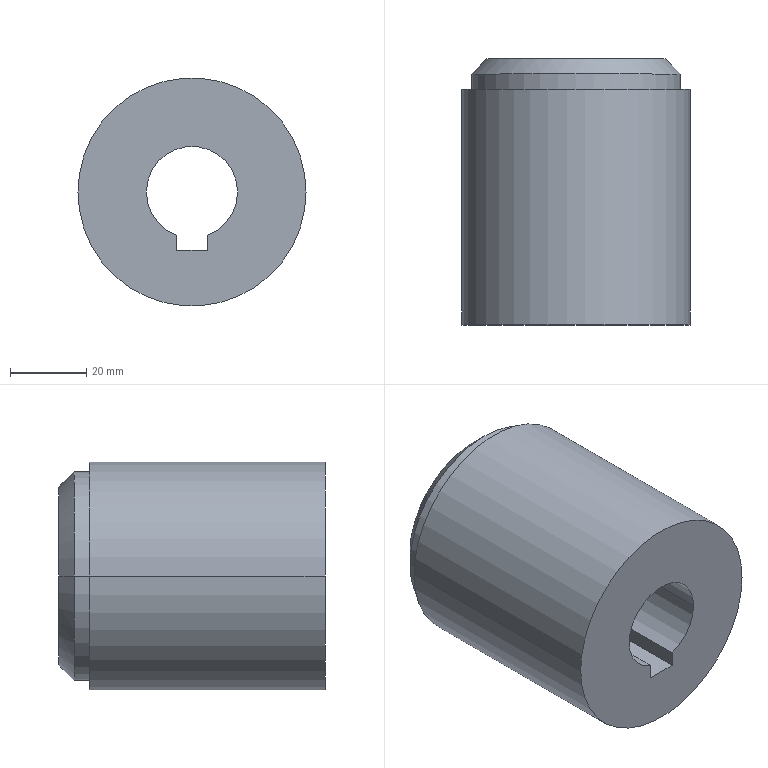Part | SolidWorks | 1 solid | 18 faces | box 60 x 70 x 60 mm | volume 151590 mm3 | cylinder 9 | plane 7 | cone 2 | commonest cylinder face diameters 24 x3 40 x2 55 x2 60 x2
STEP:
#1=CARTESIAN_POINT('',(-12.,0.,0.));
#2=VERTEX_POINT('',#1);
#3=CARTESIAN_POINT('',(-4.,0.,-11.314));
#4=VERTEX_POINT('',#3);
#5=CARTESIAN_POINT('',(0.,0.,0.));
#6=DIRECTION('',(0.,-1.,0.));
#7=DIRECTION('',(-1.,0.,0.));
#8=AXIS2_PLACEMENT_3D('',#5,#6,#7);
#9=CIRCLE('',#8,12.);
#10=EDGE_CURVE('',#2,#4,#9,.T.);
#11=ORIENTED_EDGE('',*,*,#10,.T.);
#12=CARTESIAN_POINT('',(-4.,60.,-11.314));
#13=VERTEX_POINT('',#12);
#14=CARTESIAN_POINT('',(-4.,60.,-11.314));
#15=DIRECTION('',(0.,-1.,0.));
#16=VECTOR('',#15,1000.);
#17=LINE('',#14,#16);
#18=EDGE_CURVE('',#13,#4,#17,.T.);
#19=ORIENTED_EDGE('',*,*,#18,.F.);
#20=CARTESIAN_POINT('',(-12.,60.,0.));
#21=VERTEX_POINT('',#20);
#22=CARTESIAN_POINT('',(0.,60.,0.));
#23=DIRECTION('',(0.,1.,0.));
#24=DIRECTION('',(-0.3333,0.,-0.9428));
#25=AXIS2_PLACEMENT_3D('',#22,#23,#24);
#26=CIRCLE('',#25,12.);
#27=EDGE_CURVE('',#13,#21,#26,.T.);
#28=ORIENTED_EDGE('',*,*,#27,.T.);
#29=CARTESIAN_POINT('',(-12.,0.,0.));
#30=DIRECTION('',(0.,1.,0.));
#31=VECTOR('',#30,1000.);
#32=LINE('',#29,#31);
#33=EDGE_CURVE('',#2,#21,#32,.T.);
#34=ORIENTED_EDGE('',*,*,#33,.F.);
#35=EDGE_LOOP('',(#11,#19,#28,#34));
#36=FACE_OUTER_BOUND('',#35,.T.);
#37=CARTESIAN_POINT('',(0.,70.,0.));
#38=DIRECTION('',(0.,-1.,0.));
#39=DIRECTION('',(-1.,0.,0.));
#40=AXIS2_PLACEMENT_3D('',#37,#38,#39);
#41=CYLINDRICAL_SURFACE('',#40,12.);
#42=ADVANCED_FACE('',(#36),#41,.F.);
#43=CARTESIAN_POINT('',(-4.,0.,-15.3));
#44=VERTEX_POINT('',#43);
#45=CARTESIAN_POINT('',(-4.,0.,-11.314));
#46=DIRECTION('',(0.,0.,-1.));
#47=VECTOR('',#46,1000.);
#48=LINE('',#45,#47);
#49=EDGE_CURVE('',#4,#44,#48,.T.);
#50=ORIENTED_EDGE('',*,*,#49,.T.);
#51=CARTESIAN_POINT('',(-4.,60.,-15.3));
#52=VERTEX_POINT('',#51);
#53=CARTESIAN_POINT('',(-4.,0.,-15.3));
#54=DIRECTION('',(0.,1.,0.));
#55=VECTOR('',#54,1000.);
#56=LINE('',#53,#55);
#57=EDGE_CURVE('',#44,#52,#56,.T.);
#58=ORIENTED_EDGE('',*,*,#57,.T.);
#59=CARTESIAN_POINT('',(-4.,60.,-11.314));
#60=DIRECTION('',(0.,0.,-1.));
#61=VECTOR('',#60,1000.);
#62=LINE('',#59,#61);
#63=EDGE_CURVE('',#13,#52,#62,.T.);
#64=ORIENTED_EDGE('',*,*,#63,.F.);
#65=ORIENTED_EDGE('',*,*,#18,.T.);
#66=EDGE_LOOP('',(#50,#58,#64,#65));
#67=FACE_OUTER_BOUND('',#66,.T.);
#68=CARTESIAN_POINT('',(-4.,70.,-6.108));
#69=DIRECTION('',(-1.,0.,0.));
#70=DIRECTION('',(0.,0.,1.));
#71=AXIS2_PLACEMENT_3D('',#68,#69,#70);
#72=PLANE('',#71);
#73=ADVANCED_FACE('',(#67),#72,.F.);
#74=CARTESIAN_POINT('',(4.,0.,-15.3));
#75=VERTEX_POINT('',#74);
#76=CARTESIAN_POINT('',(-4.,0.,-15.3));
#77=DIRECTION('',(1.,0.,0.));
#78=VECTOR('',#77,1000.);
#79=LINE('',#76,#78);
#80=EDGE_CURVE('',#44,#75,#79,.T.);
#81=ORIENTED_EDGE('',*,*,#80,.T.);
#82=CARTESIAN_POINT('',(4.,60.,-15.3));
#83=VERTEX_POINT('',#82);
#84=CARTESIAN_POINT('',(4.,0.,-15.3));
#85=DIRECTION('',(0.,1.,0.));
#86=VECTOR('',#85,1000.);
#87=LINE('',#84,#86);
#88=EDGE_CURVE('',#75,#83,#87,.T.);
#89=ORIENTED_EDGE('',*,*,#88,.T.);
#90=CARTESIAN_POINT('',(-4.,60.,-15.3));
#91=DIRECTION('',(1.,0.,0.));
#92=VECTOR('',#91,1000.);
#93=LINE('',#90,#92);
#94=EDGE_CURVE('',#52,#83,#93,.T.);
#95=ORIENTED_EDGE('',*,*,#94,.F.);
#96=ORIENTED_EDGE('',*,*,#57,.F.);
#97=EDGE_LOOP('',(#81,#89,#95,#96));
#98=FACE_OUTER_BOUND('',#97,.T.);
#99=CARTESIAN_POINT('',(-4.,70.,-15.3));
#100=DIRECTION('',(0.,0.,-1.));
#101=DIRECTION('',(0.,-1.,0.));
#102=AXIS2_PLACEMENT_3D('',#99,#100,#101);
#103=PLANE('',#102);
#104=ADVANCED_FACE('',(#98),#103,.F.);
#105=CARTESIAN_POINT('',(4.,0.,-11.314));
#106=VERTEX_POINT('',#105);
#107=CARTESIAN_POINT('',(4.,0.,-15.3));
#108=DIRECTION('',(0.,0.,1.));
#109=VECTOR('',#108,1000.);
#110=LINE('',#107,#109);
#111=EDGE_CURVE('',#75,#106,#110,.T.);
#112=ORIENTED_EDGE('',*,*,#111,.T.);
#113=CARTESIAN_POINT('',(4.,60.,-11.314));
#114=VERTEX_POINT('',#113);
#115=CARTESIAN_POINT('',(4.,0.,-11.314));
#116=DIRECTION('',(0.,1.,0.));
#117=VECTOR('',#116,1000.);
#118=LINE('',#115,#117);
#119=EDGE_CURVE('',#106,#114,#118,.T.);
#120=ORIENTED_EDGE('',*,*,#119,.T.);
#121=CARTESIAN_POINT('',(4.,60.,-15.3));
#122=DIRECTION('',(0.,0.,1.));
#123=VECTOR('',#122,1000.);
#124=LINE('',#121,#123);
#125=EDGE_CURVE('',#83,#114,#124,.T.);
#126=ORIENTED_EDGE('',*,*,#125,.F.);
#127=ORIENTED_EDGE('',*,*,#88,.F.);
#128=EDGE_LOOP('',(#112,#120,#126,#127));
#129=FACE_OUTER_BOUND('',#128,.T.);
#130=CARTESIAN_POINT('',(4.,70.,-15.3));
#131=DIRECTION('',(1.,0.,0.));
#132=DIRECTION('',(0.,1.,0.));
#133=AXIS2_PLACEMENT_3D('',#130,#131,#132);
#134=PLANE('',#133);
#135=ADVANCED_FACE('',(#129),#134,.F.);
#136=ORIENTED_EDGE('',*,*,#119,.F.);
#137=CARTESIAN_POINT('',(12.,0.,0.));
#138=VERTEX_POINT('',#137);
#139=CARTESIAN_POINT('',(0.,0.,0.));
#140=DIRECTION('',(0.,-1.,0.));
#141=DIRECTION('',(0.3333,0.,-0.9428));
#142=AXIS2_PLACEMENT_3D('',#139,#140,#141);
#143=CIRCLE('',#142,12.);
#144=EDGE_CURVE('',#106,#138,#143,.T.);
#145=ORIENTED_EDGE('',*,*,#144,.T.);
#146=CARTESIAN_POINT('',(12.,60.,0.));
#147=VERTEX_POINT('',#146);
#148=CARTESIAN_POINT('',(12.,0.,0.));
#149=DIRECTION('',(0.,1.,0.));
#150=VECTOR('',#149,1000.);
#151=LINE('',#148,#150);
#152=EDGE_CURVE('',#138,#147,#151,.T.);
#153=ORIENTED_EDGE('',*,*,#152,.T.);
#154=CARTESIAN_POINT('',(0.,60.,0.));
#155=DIRECTION('',(0.,1.,0.));
#156=DIRECTION('',(1.,0.,0.));
#157=AXIS2_PLACEMENT_3D('',#154,#155,#156);
#158=CIRCLE('',#157,12.);
#159=EDGE_CURVE('',#147,#114,#158,.T.);
#160=ORIENTED_EDGE('',*,*,#159,.T.);
#161=EDGE_LOOP('',(#136,#145,#153,#160));
#162=FACE_OUTER_BOUND('',#161,.T.);
#163=CARTESIAN_POINT('',(0.,70.,0.));
#164=DIRECTION('',(0.,-1.,0.));
#165=DIRECTION('',(-1.,0.,0.));
#166=AXIS2_PLACEMENT_3D('',#163,#164,#165);
#167=CYLINDRICAL_SURFACE('',#166,12.);
#168=ADVANCED_FACE('',(#162),#167,.F.);
#169=CARTESIAN_POINT('',(0.,0.,0.));
#170=DIRECTION('',(0.,-1.,0.));
#171=DIRECTION('',(1.,0.,0.));
#172=AXIS2_PLACEMENT_3D('',#169,#170,#171);
#173=CIRCLE('',#172,12.);
#174=EDGE_CURVE('',#138,#2,#173,.T.);
#175=ORIENTED_EDGE('',*,*,#174,.T.);
#176=ORIENTED_EDGE('',*,*,#33,.T.);
#177=CARTESIAN_POINT('',(0.,60.,0.));
#178=DIRECTION('',(0.,1.,0.));
#179=DIRECTION('',(-1.,0.,0.));
#180=AXIS2_PLACEMENT_3D('',#177,#178,#179);
#181=CIRCLE('',#180,12.);
#182=EDGE_CURVE('',#21,#147,#181,.T.);
#183=ORIENTED_EDGE('',*,*,#182,.T.);
#184=ORIENTED_EDGE('',*,*,#152,.F.);
#185=EDGE_LOOP('',(#175,#176,#183,#184));
#186=FACE_OUTER_BOUND('',#185,.T.);
#187=CARTESIAN_POINT('',(0.,70.,0.));
#188=DIRECTION('',(0.,-1.,0.));
#189=DIRECTION('',(-1.,0.,0.));
#190=AXIS2_PLACEMENT_3D('',#187,#188,#189);
#191=CYLINDRICAL_SURFACE('',#190,12.);
#192=ADVANCED_FACE('',(#186),#191,.F.);
#193=ORIENTED_EDGE('',*,*,#144,.F.);
#194=ORIENTED_EDGE('',*,*,#111,.F.);
#195=ORIENTED_EDGE('',*,*,#80,.F.);
#196=ORIENTED_EDGE('',*,*,#49,.F.);
#197=ORIENTED_EDGE('',*,*,#10,.F.);
#198=ORIENTED_EDGE('',*,*,#174,.F.);
#199=EDGE_LOOP('',(#193,#194,#195,#196,#197,#198));
#200=FACE_BOUND('',#199,.T.);
#201=CARTESIAN_POINT('',(-30.,0.,0.));
#202=VERTEX_POINT('',#201);
#203=CARTESIAN_POINT('',(30.,0.,0.));
#204=VERTEX_POINT('',#203);
#205=CARTESIAN_POINT('',(0.,0.,0.));
#206=DIRECTION('',(0.,1.,0.));
#207=DIRECTION('',(-1.,0.,0.));
#208=AXIS2_PLACEMENT_3D('',#205,#206,#207);
#209=CIRCLE('',#208,30.);
#210=EDGE_CURVE('',#202,#204,#209,.T.);
#211=ORIENTED_EDGE('',*,*,#210,.F.);
#212=CARTESIAN_POINT('',(0.,0.,0.));
#213=DIRECTION('',(0.,1.,0.));
#214=DIRECTION('',(1.,0.,0.));
#215=AXIS2_PLACEMENT_3D('',#212,#213,#214);
#216=CIRCLE('',#215,30.);
#217=EDGE_CURVE('',#204,#202,#216,.T.);
#218=ORIENTED_EDGE('',*,*,#217,.F.);
#219=EDGE_LOOP('',(#211,#218));
#220=FACE_OUTER_BOUND('',#219,.T.);
#221=CARTESIAN_POINT('',(0.,0.,0.));
#222=DIRECTION('',(0.,1.,0.));
#223=DIRECTION('',(1.,0.,0.));
#224=AXIS2_PLACEMENT_3D('',#221,#222,#223);
#225=PLANE('',#224);
#226=ADVANCED_FACE('',(#200,#220),#225,.F.);
#227=CARTESIAN_POINT('',(30.,62.,0.));
#228=VERTEX_POINT('',#227);
#229=CARTESIAN_POINT('',(30.,62.,0.));
#230=DIRECTION('',(0.,-1.,0.));
#231=VECTOR('',#230,1000.);
#232=LINE('',#229,#231);
#233=EDGE_CURVE('',#228,#204,#232,.T.);
#234=ORIENTED_EDGE('',*,*,#233,.F.);
#235=CARTESIAN_POINT('',(-30.,62.,0.));
#236=VERTEX_POINT('',#235);
#237=CARTESIAN_POINT('',(0.,62.,0.));
#238=DIRECTION('',(0.,-1.,0.));
#239=DIRECTION('',(1.,0.,0.));
#240=AXIS2_PLACEMENT_3D('',#237,#238,#239);
#241=CIRCLE('',#240,30.);
#242=EDGE_CURVE('',#228,#236,#241,.T.);
#243=ORIENTED_EDGE('',*,*,#242,.T.);
#244=CARTESIAN_POINT('',(-30.,62.,0.));
#245=DIRECTION('',(0.,-1.,0.));
#246=VECTOR('',#245,1000.);
#247=LINE('',#244,#246);
#248=EDGE_CURVE('',#236,#202,#247,.T.);
#249=ORIENTED_EDGE('',*,*,#248,.T.);
#250=ORIENTED_EDGE('',*,*,#210,.T.);
#251=EDGE_LOOP('',(#234,#243,#249,#250));
#252=FACE_OUTER_BOUND('',#251,.T.);
#253=CARTESIAN_POINT('',(0.,0.,0.));
#254=DIRECTION('',(0.,1.,0.));
#255=DIRECTION('',(1.,0.,0.));
#256=AXIS2_PLACEMENT_3D('',#253,#254,#255);
#257=CYLINDRICAL_SURFACE('',#256,30.);
#258=ADVANCED_FACE('',(#252),#257,.T.);
#259=CARTESIAN_POINT('',(0.,62.,0.));
#260=DIRECTION('',(0.,-1.,0.));
#261=DIRECTION('',(-1.,0.,0.));
#262=AXIS2_PLACEMENT_3D('',#259,#260,#261);
#263=CIRCLE('',#262,30.);
#264=EDGE_CURVE('',#236,#228,#263,.T.);
#265=ORIENTED_EDGE('',*,*,#264,.T.);
#266=ORIENTED_EDGE('',*,*,#233,.T.);
#267=ORIENTED_EDGE('',*,*,#217,.T.);
#268=ORIENTED_EDGE('',*,*,#248,.F.);
#269=EDGE_LOOP('',(#265,#266,#267,#268));
#270=FACE_OUTER_BOUND('',#269,.T.);
#271=CARTESIAN_POINT('',(0.,0.,0.));
#272=DIRECTION('',(0.,1.,0.));
#273=DIRECTION('',(1.,0.,0.));
#274=AXIS2_PLACEMENT_3D('',#271,#272,#273);
#275=CYLINDRICAL_SURFACE('',#274,30.);
#276=ADVANCED_FACE('',(#270),#275,.T.);
#277=CARTESIAN_POINT('',(-27.5,62.,0.));
#278=VERTEX_POINT('',#277);
#279=CARTESIAN_POINT('',(27.5,62.,0.));
#280=VERTEX_POINT('',#279);
#281=CARTESIAN_POINT('',(0.,62.,0.));
#282=DIRECTION('',(0.,1.,0.));
#283=DIRECTION('',(-1.,0.,0.));
#284=AXIS2_PLACEMENT_3D('',#281,#282,#283);
#285=CIRCLE('',#284,27.5);
#286=EDGE_CURVE('',#278,#280,#285,.T.);
#287=ORIENTED_EDGE('',*,*,#286,.F.);
#288=CARTESIAN_POINT('',(0.,62.,0.));
#289=DIRECTION('',(0.,1.,0.));
#290=DIRECTION('',(1.,0.,0.));
#291=AXIS2_PLACEMENT_3D('',#288,#289,#290);
#292=CIRCLE('',#291,27.5);
#293=EDGE_CURVE('',#280,#278,#292,.T.);
#294=ORIENTED_EDGE('',*,*,#293,.F.);
#295=EDGE_LOOP('',(#287,#294));
#296=FACE_BOUND('',#295,.T.);
#297=ORIENTED_EDGE('',*,*,#242,.F.);
#298=ORIENTED_EDGE('',*,*,#264,.F.);
#299=EDGE_LOOP('',(#297,#298));
#300=FACE_OUTER_BOUND('',#299,.T.);
#301=CARTESIAN_POINT('',(0.,62.,0.));
#302=DIRECTION('',(0.,1.,0.));
#303=DIRECTION('',(1.,0.,0.));
#304=AXIS2_PLACEMENT_3D('',#301,#302,#303);
#305=PLANE('',#304);
#306=ADVANCED_FACE('',(#296,#300),#305,.T.);
#307=CARTESIAN_POINT('',(-27.5,66.,0.));
#308=VERTEX_POINT('',#307);
#309=CARTESIAN_POINT('',(-27.5,62.,0.));
#310=DIRECTION('',(0.,1.,0.));
#311=VECTOR('',#310,1000.);
#312=LINE('',#309,#311);
#313=EDGE_CURVE('',#278,#308,#312,.T.);
#314=ORIENTED_EDGE('',*,*,#313,.F.);
#315=ORIENTED_EDGE('',*,*,#286,.T.);
#316=CARTESIAN_POINT('',(27.5,66.,0.));
#317=VERTEX_POINT('',#316);
#318=CARTESIAN_POINT('',(27.5,62.,0.));
#319=DIRECTION('',(0.,1.,0.));
#320=VECTOR('',#319,1000.);
#321=LINE('',#318,#320);
#322=EDGE_CURVE('',#280,#317,#321,.T.);
#323=ORIENTED_EDGE('',*,*,#322,.T.);
#324=CARTESIAN_POINT('',(0.,66.,0.));
#325=DIRECTION('',(0.,-1.,0.));
#326=DIRECTION('',(1.,0.,0.));
#327=AXIS2_PLACEMENT_3D('',#324,#325,#326);
#328=CIRCLE('',#327,27.5);
#329=EDGE_CURVE('',#317,#308,#328,.T.);
#330=ORIENTED_EDGE('',*,*,#329,.T.);
#331=EDGE_LOOP('',(#314,#315,#323,#330));
#332=FACE_OUTER_BOUND('',#331,.T.);
#333=CARTESIAN_POINT('',(0.,70.,0.));
#334=DIRECTION('',(0.,-1.,0.));
#335=DIRECTION('',(-1.,0.,0.));
#336=AXIS2_PLACEMENT_3D('',#333,#334,#335);
#337=CYLINDRICAL_SURFACE('',#336,27.5);
#338=ADVANCED_FACE('',(#332),#337,.T.);
#339=ORIENTED_EDGE('',*,*,#293,.T.);
#340=ORIENTED_EDGE('',*,*,#313,.T.);
#341=CARTESIAN_POINT('',(0.,66.,0.));
#342=DIRECTION('',(0.,-1.,0.));
#343=DIRECTION('',(-1.,0.,0.));
#344=AXIS2_PLACEMENT_3D('',#341,#342,#343);
#345=CIRCLE('',#344,27.5);
#346=EDGE_CURVE('',#308,#317,#345,.T.);
#347=ORIENTED_EDGE('',*,*,#346,.T.);
#348=ORIENTED_EDGE('',*,*,#322,.F.);
#349=EDGE_LOOP('',(#339,#340,#347,#348));
#350=FACE_OUTER_BOUND('',#349,.T.);
#351=CARTESIAN_POINT('',(0.,70.,0.));
#352=DIRECTION('',(0.,-1.,0.));
#353=DIRECTION('',(-1.,0.,0.));
#354=AXIS2_PLACEMENT_3D('',#351,#352,#353);
#355=CYLINDRICAL_SURFACE('',#354,27.5);
#356=ADVANCED_FACE('',(#350),#355,.T.);
#357=ORIENTED_EDGE('',*,*,#346,.F.);
#358=CARTESIAN_POINT('',(-23.5,70.,0.));
#359=VERTEX_POINT('',#358);
#360=CARTESIAN_POINT('',(-27.5,66.,0.));
#361=DIRECTION('',(0.7071,0.7071,0.));
#362=VECTOR('',#361,1000.);
#363=LINE('',#360,#362);
#364=EDGE_CURVE('',#308,#359,#363,.T.);
#365=ORIENTED_EDGE('',*,*,#364,.T.);
#366=CARTESIAN_POINT('',(23.5,70.,0.));
#367=VERTEX_POINT('',#366);
#368=CARTESIAN_POINT('',(0.,70.,0.));
#369=DIRECTION('',(0.,-1.,0.));
#370=DIRECTION('',(-1.,0.,0.));
#371=AXIS2_PLACEMENT_3D('',#368,#369,#370);
#372=CIRCLE('',#371,23.5);
#373=EDGE_CURVE('',#359,#367,#372,.T.);
#374=ORIENTED_EDGE('',*,*,#373,.T.);
#375=CARTESIAN_POINT('',(27.5,66.,0.));
#376=DIRECTION('',(-0.7071,0.7071,0.));
#377=VECTOR('',#376,1000.);
#378=LINE('',#375,#377);
#379=EDGE_CURVE('',#317,#367,#378,.T.);
#380=ORIENTED_EDGE('',*,*,#379,.F.);
#381=EDGE_LOOP('',(#357,#365,#374,#380));
#382=FACE_OUTER_BOUND('',#381,.T.);
#383=CARTESIAN_POINT('',(0.,70.093,0.));
#384=DIRECTION('',(0.,-1.,0.));
#385=DIRECTION('',(-1.,0.,0.));
#386=AXIS2_PLACEMENT_3D('',#383,#384,#385);
#387=CONICAL_SURFACE('',#386,23.407,0.7854);
#388=ADVANCED_FACE('',(#382),#387,.T.);
#389=ORIENTED_EDGE('',*,*,#364,.F.);
#390=ORIENTED_EDGE('',*,*,#329,.F.);
#391=ORIENTED_EDGE('',*,*,#379,.T.);
#392=CARTESIAN_POINT('',(0.,70.,0.));
#393=DIRECTION('',(0.,-1.,0.));
#394=DIRECTION('',(1.,0.,0.));
#395=AXIS2_PLACEMENT_3D('',#392,#393,#394);
#396=CIRCLE('',#395,23.5);
#397=EDGE_CURVE('',#367,#359,#396,.T.);
#398=ORIENTED_EDGE('',*,*,#397,.T.);
#399=EDGE_LOOP('',(#389,#390,#391,#398));
#400=FACE_OUTER_BOUND('',#399,.T.);
#401=CARTESIAN_POINT('',(0.,70.093,0.));
#402=DIRECTION('',(0.,-1.,0.));
#403=DIRECTION('',(-1.,0.,0.));
#404=AXIS2_PLACEMENT_3D('',#401,#402,#403);
#405=CONICAL_SURFACE('',#404,23.407,0.7854);
#406=ADVANCED_FACE('',(#400),#405,.T.);
#407=CARTESIAN_POINT('',(20.,70.,0.));
#408=VERTEX_POINT('',#407);
#409=CARTESIAN_POINT('',(-20.,70.,0.));
#410=VERTEX_POINT('',#409);
#411=CARTESIAN_POINT('',(0.,70.,0.));
#412=DIRECTION('',(0.,1.,0.));
#413=DIRECTION('',(1.,0.,0.));
#414=AXIS2_PLACEMENT_3D('',#411,#412,#413);
#415=CIRCLE('',#414,20.);
#416=EDGE_CURVE('',#408,#410,#415,.T.);
#417=ORIENTED_EDGE('',*,*,#416,.F.);
#418=CARTESIAN_POINT('',(0.,70.,0.));
#419=DIRECTION('',(0.,1.,0.));
#420=DIRECTION('',(-1.,0.,0.));
#421=AXIS2_PLACEMENT_3D('',#418,#419,#420);
#422=CIRCLE('',#421,20.);
#423=EDGE_CURVE('',#410,#408,#422,.T.);
#424=ORIENTED_EDGE('',*,*,#423,.F.);
#425=EDGE_LOOP('',(#417,#424));
#426=FACE_BOUND('',#425,.T.);
#427=ORIENTED_EDGE('',*,*,#373,.F.);
#428=ORIENTED_EDGE('',*,*,#397,.F.);
#429=EDGE_LOOP('',(#427,#428));
#430=FACE_OUTER_BOUND('',#429,.T.);
#431=CARTESIAN_POINT('',(0.,70.,0.));
#432=DIRECTION('',(0.,1.,0.));
#433=DIRECTION('',(1.,0.,0.));
#434=AXIS2_PLACEMENT_3D('',#431,#432,#433);
#435=PLANE('',#434);
#436=ADVANCED_FACE('',(#426,#430),#435,.T.);
#437=CARTESIAN_POINT('',(-20.,60.,0.));
#438=VERTEX_POINT('',#437);
#439=CARTESIAN_POINT('',(-20.,60.,0.));
#440=DIRECTION('',(0.,1.,0.));
#441=VECTOR('',#440,1000.);
#442=LINE('',#439,#441);
#443=EDGE_CURVE('',#438,#410,#442,.T.);
#444=ORIENTED_EDGE('',*,*,#443,.F.);
#445=CARTESIAN_POINT('',(20.,60.,0.));
#446=VERTEX_POINT('',#445);
#447=CARTESIAN_POINT('',(0.,60.,0.));
#448=DIRECTION('',(0.,-1.,0.));
#449=DIRECTION('',(-1.,0.,0.));
#450=AXIS2_PLACEMENT_3D('',#447,#448,#449);
#451=CIRCLE('',#450,20.);
#452=EDGE_CURVE('',#438,#446,#451,.T.);
#453=ORIENTED_EDGE('',*,*,#452,.T.);
#454=CARTESIAN_POINT('',(20.,60.,0.));
#455=DIRECTION('',(0.,1.,0.));
#456=VECTOR('',#455,1000.);
#457=LINE('',#454,#456);
#458=EDGE_CURVE('',#446,#408,#457,.T.);
#459=ORIENTED_EDGE('',*,*,#458,.T.);
#460=ORIENTED_EDGE('',*,*,#416,.T.);
#461=EDGE_LOOP('',(#444,#453,#459,#460));
#462=FACE_OUTER_BOUND('',#461,.T.);
#463=CARTESIAN_POINT('',(0.,70.,0.));
#464=DIRECTION('',(0.,-1.,0.));
#465=DIRECTION('',(-1.,0.,0.));
#466=AXIS2_PLACEMENT_3D('',#463,#464,#465);
#467=CYLINDRICAL_SURFACE('',#466,20.);
#468=ADVANCED_FACE('',(#462),#467,.F.);
#469=CARTESIAN_POINT('',(0.,60.,0.));
#470=DIRECTION('',(0.,-1.,0.));
#471=DIRECTION('',(1.,0.,0.));
#472=AXIS2_PLACEMENT_3D('',#469,#470,#471);
#473=CIRCLE('',#472,20.);
#474=EDGE_CURVE('',#446,#438,#473,.T.);
#475=ORIENTED_EDGE('',*,*,#474,.T.);
#476=ORIENTED_EDGE('',*,*,#443,.T.);
#477=ORIENTED_EDGE('',*,*,#423,.T.);
#478=ORIENTED_EDGE('',*,*,#458,.F.);
#479=EDGE_LOOP('',(#475,#476,#477,#478));
#480=FACE_OUTER_BOUND('',#479,.T.);
#481=CARTESIAN_POINT('',(0.,70.,0.));
#482=DIRECTION('',(0.,-1.,0.));
#483=DIRECTION('',(-1.,0.,0.));
#484=AXIS2_PLACEMENT_3D('',#481,#482,#483);
#485=CYLINDRICAL_SURFACE('',#484,20.);
#486=ADVANCED_FACE('',(#480),#485,.F.);
#487=ORIENTED_EDGE('',*,*,#159,.F.);
#488=ORIENTED_EDGE('',*,*,#182,.F.);
#489=ORIENTED_EDGE('',*,*,#27,.F.);
#490=ORIENTED_EDGE('',*,*,#63,.T.);
#491=ORIENTED_EDGE('',*,*,#94,.T.);
#492=ORIENTED_EDGE('',*,*,#125,.T.);
#493=EDGE_LOOP('',(#487,#488,#489,#490,#491,#492));
#494=FACE_BOUND('',#493,.T.);
#495=ORIENTED_EDGE('',*,*,#452,.F.);
#496=ORIENTED_EDGE('',*,*,#474,.F.);
#497=EDGE_LOOP('',(#495,#496));
#498=FACE_OUTER_BOUND('',#497,.T.);
#499=CARTESIAN_POINT('',(0.,60.,0.));
#500=DIRECTION('',(0.,1.,0.));
#501=DIRECTION('',(1.,0.,0.));
#502=AXIS2_PLACEMENT_3D('',#499,#500,#501);
#503=PLANE('',#502);
#504=ADVANCED_FACE('',(#494,#498),#503,.T.);
#505=CLOSED_SHELL('',(#42,#73,#104,#135,#168,#192,#226,#258,#276,#306,#338,#356,#388,#406,#436,#468,#486,#504));
#506=MANIFOLD_SOLID_BREP('',#505);
#507=CARTESIAN_POINT('',(0.,0.,0.));
#508=DIRECTION('',(0.,0.,1.));
#509=DIRECTION('',(1.,0.,0.));
#510=AXIS2_PLACEMENT_3D('',#507,#508,#509);
#511=(LENGTH_UNIT()NAMED_UNIT(*)SI_UNIT(.MILLI.,.METRE.));
#512=UNCERTAINTY_MEASURE_WITH_UNIT(LENGTH_MEASURE(0.00001),#511,'','');
#513=(NAMED_UNIT(*)PLANE_ANGLE_UNIT()SI_UNIT($,.RADIAN.));
#514=(NAMED_UNIT(*)SI_UNIT($,.STERADIAN.)SOLID_ANGLE_UNIT());
#515=(GEOMETRIC_REPRESENTATION_CONTEXT(3)GLOBAL_UNCERTAINTY_ASSIGNED_CONTEXT((#512))GLOBAL_UNIT_ASSIGNED_CONTEXT((#511,#513,#514))REPRESENTATION_CONTEXT('',''));
#516=ADVANCED_BREP_SHAPE_REPRESENTATION('',(#506,#510),#515);